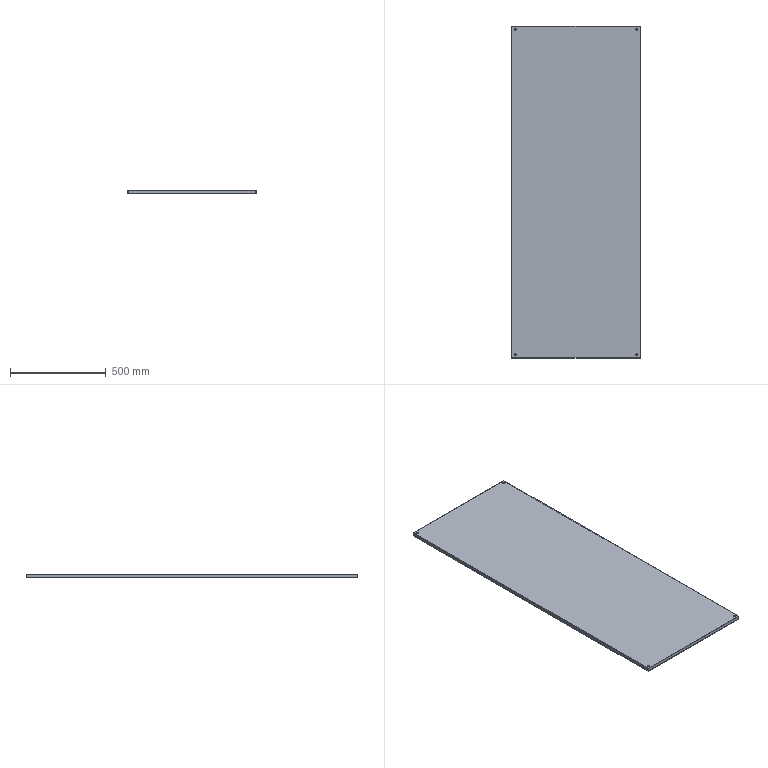Part | SolidWorks | features Extrusion 1, HoleWzd 1, ICE 1, Shell 1 | 1 solid | 32 faces | box 669 x 1734 x 20 mm | volume 2661634 mm3 | cylinder 16 | plane 16 | commonest cylinder face diameters 6.6 x8 11 x8
STEP:
#1=CARTESIAN_POINT('',(-312.,850.,18.));
#2=VERTEX_POINT('',#1);
#3=CARTESIAN_POINT('',(-323.,850.,18.));
#4=VERTEX_POINT('',#3);
#5=CARTESIAN_POINT('',(-317.5,850.,18.));
#6=DIRECTION('',(0.,0.,-1.));
#7=DIRECTION('',(-1.,0.,0.));
#8=AXIS2_PLACEMENT_3D('',#5,#6,#7);
#9=CIRCLE('',#8,5.5);
#10=EDGE_CURVE('',#2,#4,#9,.T.);
#11=ORIENTED_EDGE('',*,*,#10,.T.);
#12=CARTESIAN_POINT('',(-323.,850.,20.));
#13=VERTEX_POINT('',#12);
#14=CARTESIAN_POINT('',(-323.,850.,20.));
#15=DIRECTION('',(0.,0.,1.));
#16=VECTOR('',#15,1000.);
#17=LINE('',#14,#16);
#18=EDGE_CURVE('',#4,#13,#17,.T.);
#19=ORIENTED_EDGE('',*,*,#18,.T.);
#20=CARTESIAN_POINT('',(-312.,850.,20.));
#21=VERTEX_POINT('',#20);
#22=CARTESIAN_POINT('',(-317.5,850.,20.));
#23=DIRECTION('',(0.,0.,1.));
#24=DIRECTION('',(1.,0.,0.));
#25=AXIS2_PLACEMENT_3D('',#22,#23,#24);
#26=CIRCLE('',#25,5.5);
#27=EDGE_CURVE('',#13,#21,#26,.T.);
#28=ORIENTED_EDGE('',*,*,#27,.T.);
#29=CARTESIAN_POINT('',(-312.,850.,20.));
#30=DIRECTION('',(0.,0.,1.));
#31=VECTOR('',#30,1000.);
#32=LINE('',#29,#31);
#33=EDGE_CURVE('',#2,#21,#32,.T.);
#34=ORIENTED_EDGE('',*,*,#33,.F.);
#35=EDGE_LOOP('',(#11,#19,#28,#34));
#36=FACE_OUTER_BOUND('',#35,.T.);
#37=CARTESIAN_POINT('',(-317.5,850.,20.));
#38=DIRECTION('',(0.,0.,1.));
#39=DIRECTION('',(1.,0.,0.));
#40=AXIS2_PLACEMENT_3D('',#37,#38,#39);
#41=CYLINDRICAL_SURFACE('',#40,5.5);
#42=ADVANCED_FACE('',(#36),#41,.F.);
#43=CARTESIAN_POINT('',(-320.8,850.,0.));
#44=VERTEX_POINT('',#43);
#45=CARTESIAN_POINT('',(-314.2,850.,0.));
#46=VERTEX_POINT('',#45);
#47=CARTESIAN_POINT('',(-317.5,850.,0.));
#48=DIRECTION('',(0.,0.,1.));
#49=DIRECTION('',(1.,0.,0.));
#50=AXIS2_PLACEMENT_3D('',#47,#48,#49);
#51=CIRCLE('',#50,3.3);
#52=EDGE_CURVE('',#44,#46,#51,.T.);
#53=ORIENTED_EDGE('',*,*,#52,.F.);
#54=CARTESIAN_POINT('',(-320.8,850.,2.));
#55=VERTEX_POINT('',#54);
#56=CARTESIAN_POINT('',(-320.8,850.,20.));
#57=DIRECTION('',(0.,0.,1.));
#58=VECTOR('',#57,1000.);
#59=LINE('',#56,#58);
#60=EDGE_CURVE('',#44,#55,#59,.T.);
#61=ORIENTED_EDGE('',*,*,#60,.T.);
#62=CARTESIAN_POINT('',(-314.2,850.,2.));
#63=VERTEX_POINT('',#62);
#64=CARTESIAN_POINT('',(-317.5,850.,2.));
#65=DIRECTION('',(0.,0.,-1.));
#66=DIRECTION('',(-1.,0.,0.));
#67=AXIS2_PLACEMENT_3D('',#64,#65,#66);
#68=CIRCLE('',#67,3.3);
#69=EDGE_CURVE('',#63,#55,#68,.T.);
#70=ORIENTED_EDGE('',*,*,#69,.F.);
#71=CARTESIAN_POINT('',(-314.2,850.,20.));
#72=DIRECTION('',(0.,0.,1.));
#73=VECTOR('',#72,1000.);
#74=LINE('',#71,#73);
#75=EDGE_CURVE('',#46,#63,#74,.T.);
#76=ORIENTED_EDGE('',*,*,#75,.F.);
#77=EDGE_LOOP('',(#53,#61,#70,#76));
#78=FACE_OUTER_BOUND('',#77,.T.);
#79=CARTESIAN_POINT('',(-317.5,850.,20.));
#80=DIRECTION('',(0.,0.,1.));
#81=DIRECTION('',(1.,0.,0.));
#82=AXIS2_PLACEMENT_3D('',#79,#80,#81);
#83=CYLINDRICAL_SURFACE('',#82,3.3);
#84=ADVANCED_FACE('',(#78),#83,.F.);
#85=CARTESIAN_POINT('',(-312.,-850.,18.));
#86=VERTEX_POINT('',#85);
#87=CARTESIAN_POINT('',(-323.,-850.,18.));
#88=VERTEX_POINT('',#87);
#89=CARTESIAN_POINT('',(-317.5,-850.,18.));
#90=DIRECTION('',(0.,0.,-1.));
#91=DIRECTION('',(-1.,0.,0.));
#92=AXIS2_PLACEMENT_3D('',#89,#90,#91);
#93=CIRCLE('',#92,5.5);
#94=EDGE_CURVE('',#86,#88,#93,.T.);
#95=ORIENTED_EDGE('',*,*,#94,.T.);
#96=CARTESIAN_POINT('',(-323.,-850.,20.));
#97=VERTEX_POINT('',#96);
#98=CARTESIAN_POINT('',(-323.,-850.,20.));
#99=DIRECTION('',(0.,0.,1.));
#100=VECTOR('',#99,1000.);
#101=LINE('',#98,#100);
#102=EDGE_CURVE('',#88,#97,#101,.T.);
#103=ORIENTED_EDGE('',*,*,#102,.T.);
#104=CARTESIAN_POINT('',(-312.,-850.,20.));
#105=VERTEX_POINT('',#104);
#106=CARTESIAN_POINT('',(-317.5,-850.,20.));
#107=DIRECTION('',(0.,0.,1.));
#108=DIRECTION('',(1.,0.,0.));
#109=AXIS2_PLACEMENT_3D('',#106,#107,#108);
#110=CIRCLE('',#109,5.5);
#111=EDGE_CURVE('',#97,#105,#110,.T.);
#112=ORIENTED_EDGE('',*,*,#111,.T.);
#113=CARTESIAN_POINT('',(-312.,-850.,20.));
#114=DIRECTION('',(0.,0.,1.));
#115=VECTOR('',#114,1000.);
#116=LINE('',#113,#115);
#117=EDGE_CURVE('',#86,#105,#116,.T.);
#118=ORIENTED_EDGE('',*,*,#117,.F.);
#119=EDGE_LOOP('',(#95,#103,#112,#118));
#120=FACE_OUTER_BOUND('',#119,.T.);
#121=CARTESIAN_POINT('',(-317.5,-850.,20.));
#122=DIRECTION('',(0.,0.,1.));
#123=DIRECTION('',(1.,0.,0.));
#124=AXIS2_PLACEMENT_3D('',#121,#122,#123);
#125=CYLINDRICAL_SURFACE('',#124,5.5);
#126=ADVANCED_FACE('',(#120),#125,.F.);
#127=CARTESIAN_POINT('',(-320.8,-850.,0.));
#128=VERTEX_POINT('',#127);
#129=CARTESIAN_POINT('',(-314.2,-850.,0.));
#130=VERTEX_POINT('',#129);
#131=CARTESIAN_POINT('',(-317.5,-850.,0.));
#132=DIRECTION('',(0.,0.,1.));
#133=DIRECTION('',(1.,0.,0.));
#134=AXIS2_PLACEMENT_3D('',#131,#132,#133);
#135=CIRCLE('',#134,3.3);
#136=EDGE_CURVE('',#128,#130,#135,.T.);
#137=ORIENTED_EDGE('',*,*,#136,.F.);
#138=CARTESIAN_POINT('',(-320.8,-850.,2.));
#139=VERTEX_POINT('',#138);
#140=CARTESIAN_POINT('',(-320.8,-850.,20.));
#141=DIRECTION('',(0.,0.,1.));
#142=VECTOR('',#141,1000.);
#143=LINE('',#140,#142);
#144=EDGE_CURVE('',#128,#139,#143,.T.);
#145=ORIENTED_EDGE('',*,*,#144,.T.);
#146=CARTESIAN_POINT('',(-314.2,-850.,2.));
#147=VERTEX_POINT('',#146);
#148=CARTESIAN_POINT('',(-317.5,-850.,2.));
#149=DIRECTION('',(0.,0.,-1.));
#150=DIRECTION('',(-1.,0.,0.));
#151=AXIS2_PLACEMENT_3D('',#148,#149,#150);
#152=CIRCLE('',#151,3.3);
#153=EDGE_CURVE('',#147,#139,#152,.T.);
#154=ORIENTED_EDGE('',*,*,#153,.F.);
#155=CARTESIAN_POINT('',(-314.2,-850.,20.));
#156=DIRECTION('',(0.,0.,1.));
#157=VECTOR('',#156,1000.);
#158=LINE('',#155,#157);
#159=EDGE_CURVE('',#130,#147,#158,.T.);
#160=ORIENTED_EDGE('',*,*,#159,.F.);
#161=EDGE_LOOP('',(#137,#145,#154,#160));
#162=FACE_OUTER_BOUND('',#161,.T.);
#163=CARTESIAN_POINT('',(-317.5,-850.,20.));
#164=DIRECTION('',(0.,0.,1.));
#165=DIRECTION('',(1.,0.,0.));
#166=AXIS2_PLACEMENT_3D('',#163,#164,#165);
#167=CYLINDRICAL_SURFACE('',#166,3.3);
#168=ADVANCED_FACE('',(#162),#167,.F.);
#169=CARTESIAN_POINT('',(314.2,-850.,0.));
#170=VERTEX_POINT('',#169);
#171=CARTESIAN_POINT('',(320.8,-850.,0.));
#172=VERTEX_POINT('',#171);
#173=CARTESIAN_POINT('',(317.5,-850.,0.));
#174=DIRECTION('',(0.,0.,1.));
#175=DIRECTION('',(1.,0.,0.));
#176=AXIS2_PLACEMENT_3D('',#173,#174,#175);
#177=CIRCLE('',#176,3.3);
#178=EDGE_CURVE('',#170,#172,#177,.T.);
#179=ORIENTED_EDGE('',*,*,#178,.F.);
#180=CARTESIAN_POINT('',(314.2,-850.,2.));
#181=VERTEX_POINT('',#180);
#182=CARTESIAN_POINT('',(314.2,-850.,20.));
#183=DIRECTION('',(0.,0.,1.));
#184=VECTOR('',#183,1000.);
#185=LINE('',#182,#184);
#186=EDGE_CURVE('',#170,#181,#185,.T.);
#187=ORIENTED_EDGE('',*,*,#186,.T.);
#188=CARTESIAN_POINT('',(320.8,-850.,2.));
#189=VERTEX_POINT('',#188);
#190=CARTESIAN_POINT('',(317.5,-850.,2.));
#191=DIRECTION('',(0.,0.,-1.));
#192=DIRECTION('',(-1.,0.,0.));
#193=AXIS2_PLACEMENT_3D('',#190,#191,#192);
#194=CIRCLE('',#193,3.3);
#195=EDGE_CURVE('',#189,#181,#194,.T.);
#196=ORIENTED_EDGE('',*,*,#195,.F.);
#197=CARTESIAN_POINT('',(320.8,-850.,20.));
#198=DIRECTION('',(0.,0.,1.));
#199=VECTOR('',#198,1000.);
#200=LINE('',#197,#199);
#201=EDGE_CURVE('',#172,#189,#200,.T.);
#202=ORIENTED_EDGE('',*,*,#201,.F.);
#203=EDGE_LOOP('',(#179,#187,#196,#202));
#204=FACE_OUTER_BOUND('',#203,.T.);
#205=CARTESIAN_POINT('',(317.5,-850.,20.));
#206=DIRECTION('',(0.,0.,1.));
#207=DIRECTION('',(1.,0.,0.));
#208=AXIS2_PLACEMENT_3D('',#205,#206,#207);
#209=CYLINDRICAL_SURFACE('',#208,3.3);
#210=ADVANCED_FACE('',(#204),#209,.F.);
#211=CARTESIAN_POINT('',(323.,-850.,18.));
#212=VERTEX_POINT('',#211);
#213=CARTESIAN_POINT('',(312.,-850.,18.));
#214=VERTEX_POINT('',#213);
#215=CARTESIAN_POINT('',(317.5,-850.,18.));
#216=DIRECTION('',(0.,0.,-1.));
#217=DIRECTION('',(-1.,0.,0.));
#218=AXIS2_PLACEMENT_3D('',#215,#216,#217);
#219=CIRCLE('',#218,5.5);
#220=EDGE_CURVE('',#212,#214,#219,.T.);
#221=ORIENTED_EDGE('',*,*,#220,.T.);
#222=CARTESIAN_POINT('',(312.,-850.,20.));
#223=VERTEX_POINT('',#222);
#224=CARTESIAN_POINT('',(312.,-850.,20.));
#225=DIRECTION('',(0.,0.,1.));
#226=VECTOR('',#225,1000.);
#227=LINE('',#224,#226);
#228=EDGE_CURVE('',#214,#223,#227,.T.);
#229=ORIENTED_EDGE('',*,*,#228,.T.);
#230=CARTESIAN_POINT('',(323.,-850.,20.));
#231=VERTEX_POINT('',#230);
#232=CARTESIAN_POINT('',(317.5,-850.,20.));
#233=DIRECTION('',(0.,0.,1.));
#234=DIRECTION('',(1.,0.,0.));
#235=AXIS2_PLACEMENT_3D('',#232,#233,#234);
#236=CIRCLE('',#235,5.5);
#237=EDGE_CURVE('',#223,#231,#236,.T.);
#238=ORIENTED_EDGE('',*,*,#237,.T.);
#239=CARTESIAN_POINT('',(323.,-850.,20.));
#240=DIRECTION('',(0.,0.,1.));
#241=VECTOR('',#240,1000.);
#242=LINE('',#239,#241);
#243=EDGE_CURVE('',#212,#231,#242,.T.);
#244=ORIENTED_EDGE('',*,*,#243,.F.);
#245=EDGE_LOOP('',(#221,#229,#238,#244));
#246=FACE_OUTER_BOUND('',#245,.T.);
#247=CARTESIAN_POINT('',(317.5,-850.,20.));
#248=DIRECTION('',(0.,0.,1.));
#249=DIRECTION('',(1.,0.,0.));
#250=AXIS2_PLACEMENT_3D('',#247,#248,#249);
#251=CYLINDRICAL_SURFACE('',#250,5.5);
#252=ADVANCED_FACE('',(#246),#251,.F.);
#253=CARTESIAN_POINT('',(314.2,850.,0.));
#254=VERTEX_POINT('',#253);
#255=CARTESIAN_POINT('',(320.8,850.,0.));
#256=VERTEX_POINT('',#255);
#257=CARTESIAN_POINT('',(317.5,850.,0.));
#258=DIRECTION('',(0.,0.,1.));
#259=DIRECTION('',(1.,0.,0.));
#260=AXIS2_PLACEMENT_3D('',#257,#258,#259);
#261=CIRCLE('',#260,3.3);
#262=EDGE_CURVE('',#254,#256,#261,.T.);
#263=ORIENTED_EDGE('',*,*,#262,.F.);
#264=CARTESIAN_POINT('',(314.2,850.,2.));
#265=VERTEX_POINT('',#264);
#266=CARTESIAN_POINT('',(314.2,850.,20.));
#267=DIRECTION('',(0.,0.,1.));
#268=VECTOR('',#267,1000.);
#269=LINE('',#266,#268);
#270=EDGE_CURVE('',#254,#265,#269,.T.);
#271=ORIENTED_EDGE('',*,*,#270,.T.);
#272=CARTESIAN_POINT('',(320.8,850.,2.));
#273=VERTEX_POINT('',#272);
#274=CARTESIAN_POINT('',(317.5,850.,2.));
#275=DIRECTION('',(0.,0.,-1.));
#276=DIRECTION('',(-1.,0.,0.));
#277=AXIS2_PLACEMENT_3D('',#274,#275,#276);
#278=CIRCLE('',#277,3.3);
#279=EDGE_CURVE('',#273,#265,#278,.T.);
#280=ORIENTED_EDGE('',*,*,#279,.F.);
#281=CARTESIAN_POINT('',(320.8,850.,20.));
#282=DIRECTION('',(0.,0.,1.));
#283=VECTOR('',#282,1000.);
#284=LINE('',#281,#283);
#285=EDGE_CURVE('',#256,#273,#284,.T.);
#286=ORIENTED_EDGE('',*,*,#285,.F.);
#287=EDGE_LOOP('',(#263,#271,#280,#286));
#288=FACE_OUTER_BOUND('',#287,.T.);
#289=CARTESIAN_POINT('',(317.5,850.,20.));
#290=DIRECTION('',(0.,0.,1.));
#291=DIRECTION('',(1.,0.,0.));
#292=AXIS2_PLACEMENT_3D('',#289,#290,#291);
#293=CYLINDRICAL_SURFACE('',#292,3.3);
#294=ADVANCED_FACE('',(#288),#293,.F.);
#295=CARTESIAN_POINT('',(323.,850.,18.));
#296=VERTEX_POINT('',#295);
#297=CARTESIAN_POINT('',(312.,850.,18.));
#298=VERTEX_POINT('',#297);
#299=CARTESIAN_POINT('',(317.5,850.,18.));
#300=DIRECTION('',(0.,0.,-1.));
#301=DIRECTION('',(-1.,0.,0.));
#302=AXIS2_PLACEMENT_3D('',#299,#300,#301);
#303=CIRCLE('',#302,5.5);
#304=EDGE_CURVE('',#296,#298,#303,.T.);
#305=ORIENTED_EDGE('',*,*,#304,.T.);
#306=CARTESIAN_POINT('',(312.,850.,20.));
#307=VERTEX_POINT('',#306);
#308=CARTESIAN_POINT('',(312.,850.,20.));
#309=DIRECTION('',(0.,0.,1.));
#310=VECTOR('',#309,1000.);
#311=LINE('',#308,#310);
#312=EDGE_CURVE('',#298,#307,#311,.T.);
#313=ORIENTED_EDGE('',*,*,#312,.T.);
#314=CARTESIAN_POINT('',(323.,850.,20.));
#315=VERTEX_POINT('',#314);
#316=CARTESIAN_POINT('',(317.5,850.,20.));
#317=DIRECTION('',(0.,0.,1.));
#318=DIRECTION('',(1.,0.,0.));
#319=AXIS2_PLACEMENT_3D('',#316,#317,#318);
#320=CIRCLE('',#319,5.5);
#321=EDGE_CURVE('',#307,#315,#320,.T.);
#322=ORIENTED_EDGE('',*,*,#321,.T.);
#323=CARTESIAN_POINT('',(323.,850.,20.));
#324=DIRECTION('',(0.,0.,1.));
#325=VECTOR('',#324,1000.);
#326=LINE('',#323,#325);
#327=EDGE_CURVE('',#296,#315,#326,.T.);
#328=ORIENTED_EDGE('',*,*,#327,.F.);
#329=EDGE_LOOP('',(#305,#313,#322,#328));
#330=FACE_OUTER_BOUND('',#329,.T.);
#331=CARTESIAN_POINT('',(317.5,850.,20.));
#332=DIRECTION('',(0.,0.,1.));
#333=DIRECTION('',(1.,0.,0.));
#334=AXIS2_PLACEMENT_3D('',#331,#332,#333);
#335=CYLINDRICAL_SURFACE('',#334,5.5);
#336=ADVANCED_FACE('',(#330),#335,.F.);
#337=CARTESIAN_POINT('',(-317.5,850.,0.));
#338=DIRECTION('',(0.,0.,1.));
#339=DIRECTION('',(1.,0.,0.));
#340=AXIS2_PLACEMENT_3D('',#337,#338,#339);
#341=CIRCLE('',#340,3.3);
#342=EDGE_CURVE('',#46,#44,#341,.T.);
#343=ORIENTED_EDGE('',*,*,#342,.T.);
#344=ORIENTED_EDGE('',*,*,#52,.T.);
#345=EDGE_LOOP('',(#343,#344));
#346=FACE_BOUND('',#345,.T.);
#347=CARTESIAN_POINT('',(-317.5,-850.,0.));
#348=DIRECTION('',(0.,0.,1.));
#349=DIRECTION('',(1.,0.,0.));
#350=AXIS2_PLACEMENT_3D('',#347,#348,#349);
#351=CIRCLE('',#350,3.3);
#352=EDGE_CURVE('',#130,#128,#351,.T.);
#353=ORIENTED_EDGE('',*,*,#352,.T.);
#354=ORIENTED_EDGE('',*,*,#136,.T.);
#355=EDGE_LOOP('',(#353,#354));
#356=FACE_BOUND('',#355,.T.);
#357=CARTESIAN_POINT('',(317.5,-850.,0.));
#358=DIRECTION('',(0.,0.,1.));
#359=DIRECTION('',(1.,0.,0.));
#360=AXIS2_PLACEMENT_3D('',#357,#358,#359);
#361=CIRCLE('',#360,3.3);
#362=EDGE_CURVE('',#172,#170,#361,.T.);
#363=ORIENTED_EDGE('',*,*,#362,.T.);
#364=ORIENTED_EDGE('',*,*,#178,.T.);
#365=EDGE_LOOP('',(#363,#364));
#366=FACE_BOUND('',#365,.T.);
#367=CARTESIAN_POINT('',(317.5,850.,0.));
#368=DIRECTION('',(0.,0.,1.));
#369=DIRECTION('',(1.,0.,0.));
#370=AXIS2_PLACEMENT_3D('',#367,#368,#369);
#371=CIRCLE('',#370,3.3);
#372=EDGE_CURVE('',#256,#254,#371,.T.);
#373=ORIENTED_EDGE('',*,*,#372,.T.);
#374=ORIENTED_EDGE('',*,*,#262,.T.);
#375=EDGE_LOOP('',(#373,#374));
#376=FACE_BOUND('',#375,.T.);
#377=CARTESIAN_POINT('',(334.5,-867.,0.));
#378=VERTEX_POINT('',#377);
#379=CARTESIAN_POINT('',(334.5,867.,0.));
#380=VERTEX_POINT('',#379);
#381=CARTESIAN_POINT('',(334.5,-867.,0.));
#382=DIRECTION('',(0.,1.,0.));
#383=VECTOR('',#382,1000.);
#384=LINE('',#381,#383);
#385=EDGE_CURVE('',#378,#380,#384,.T.);
#386=ORIENTED_EDGE('',*,*,#385,.F.);
#387=CARTESIAN_POINT('',(-334.5,-867.,0.));
#388=VERTEX_POINT('',#387);
#389=CARTESIAN_POINT('',(-334.5,-867.,0.));
#390=DIRECTION('',(1.,0.,0.));
#391=VECTOR('',#390,1000.);
#392=LINE('',#389,#391);
#393=EDGE_CURVE('',#388,#378,#392,.T.);
#394=ORIENTED_EDGE('',*,*,#393,.F.);
#395=CARTESIAN_POINT('',(-334.5,867.,0.));
#396=VERTEX_POINT('',#395);
#397=CARTESIAN_POINT('',(-334.5,-867.,0.));
#398=DIRECTION('',(0.,-1.,0.));
#399=VECTOR('',#398,1000.);
#400=LINE('',#397,#399);
#401=EDGE_CURVE('',#396,#388,#400,.T.);
#402=ORIENTED_EDGE('',*,*,#401,.F.);
#403=CARTESIAN_POINT('',(-334.5,867.,0.));
#404=DIRECTION('',(-1.,0.,0.));
#405=VECTOR('',#404,1000.);
#406=LINE('',#403,#405);
#407=EDGE_CURVE('',#380,#396,#406,.T.);
#408=ORIENTED_EDGE('',*,*,#407,.F.);
#409=EDGE_LOOP('',(#386,#394,#402,#408));
#410=FACE_OUTER_BOUND('',#409,.T.);
#411=CARTESIAN_POINT('',(314.5,-847.,0.));
#412=VERTEX_POINT('',#411);
#413=CARTESIAN_POINT('',(-314.5,-847.,0.));
#414=VERTEX_POINT('',#413);
#415=CARTESIAN_POINT('',(314.5,-847.,0.));
#416=DIRECTION('',(-1.,0.,0.));
#417=VECTOR('',#416,1000.);
#418=LINE('',#415,#417);
#419=EDGE_CURVE('',#412,#414,#418,.T.);
#420=ORIENTED_EDGE('',*,*,#419,.F.);
#421=CARTESIAN_POINT('',(314.5,847.,0.));
#422=VERTEX_POINT('',#421);
#423=CARTESIAN_POINT('',(314.5,-847.,0.));
#424=DIRECTION('',(0.,1.,0.));
#425=VECTOR('',#424,1000.);
#426=LINE('',#423,#425);
#427=EDGE_CURVE('',#412,#422,#426,.T.);
#428=ORIENTED_EDGE('',*,*,#427,.T.);
#429=CARTESIAN_POINT('',(-314.5,847.,0.));
#430=VERTEX_POINT('',#429);
#431=CARTESIAN_POINT('',(314.5,847.,0.));
#432=DIRECTION('',(-1.,0.,0.));
#433=VECTOR('',#432,1000.);
#434=LINE('',#431,#433);
#435=EDGE_CURVE('',#422,#430,#434,.T.);
#436=ORIENTED_EDGE('',*,*,#435,.T.);
#437=CARTESIAN_POINT('',(-314.5,-847.,0.));
#438=DIRECTION('',(0.,1.,0.));
#439=VECTOR('',#438,1000.);
#440=LINE('',#437,#439);
#441=EDGE_CURVE('',#414,#430,#440,.T.);
#442=ORIENTED_EDGE('',*,*,#441,.F.);
#443=EDGE_LOOP('',(#420,#428,#436,#442));
#444=FACE_BOUND('',#443,.T.);
#445=CARTESIAN_POINT('',(0.,0.,0.));
#446=DIRECTION('',(0.,0.,-1.));
#447=DIRECTION('',(-1.,0.,0.));
#448=AXIS2_PLACEMENT_3D('',#445,#446,#447);
#449=PLANE('',#448);
#450=ADVANCED_FACE('',(#346,#356,#366,#376,#410,#444),#449,.T.);
#451=ORIENTED_EDGE('',*,*,#385,.T.);
#452=CARTESIAN_POINT('',(334.5,867.,20.));
#453=VERTEX_POINT('',#452);
#454=CARTESIAN_POINT('',(334.5,867.,20.));
#455=DIRECTION('',(0.,0.,-1.));
#456=VECTOR('',#455,1000.);
#457=LINE('',#454,#456);
#458=EDGE_CURVE('',#453,#380,#457,.T.);
#459=ORIENTED_EDGE('',*,*,#458,.F.);
#460=CARTESIAN_POINT('',(334.5,-867.,20.));
#461=VERTEX_POINT('',#460);
#462=CARTESIAN_POINT('',(334.5,-867.,20.));
#463=DIRECTION('',(0.,1.,0.));
#464=VECTOR('',#463,1000.);
#465=LINE('',#462,#464);
#466=EDGE_CURVE('',#461,#453,#465,.T.);
#467=ORIENTED_EDGE('',*,*,#466,.F.);
#468=CARTESIAN_POINT('',(334.5,-867.,20.));
#469=DIRECTION('',(0.,0.,-1.));
#470=VECTOR('',#469,1000.);
#471=LINE('',#468,#470);
#472=EDGE_CURVE('',#461,#378,#471,.T.);
#473=ORIENTED_EDGE('',*,*,#472,.T.);
#474=EDGE_LOOP('',(#451,#459,#467,#473));
#475=FACE_OUTER_BOUND('',#474,.T.);
#476=CARTESIAN_POINT('',(334.5,-867.,20.));
#477=DIRECTION('',(-1.,0.,0.));
#478=DIRECTION('',(0.,0.,1.));
#479=AXIS2_PLACEMENT_3D('',#476,#477,#478);
#480=PLANE('',#479);
#481=ADVANCED_FACE('',(#475),#480,.F.);
#482=ORIENTED_EDGE('',*,*,#407,.T.);
#483=CARTESIAN_POINT('',(-334.5,867.,20.));
#484=VERTEX_POINT('',#483);
#485=CARTESIAN_POINT('',(-334.5,867.,20.));
#486=DIRECTION('',(0.,0.,-1.));
#487=VECTOR('',#486,1000.);
#488=LINE('',#485,#487);
#489=EDGE_CURVE('',#484,#396,#488,.T.);
#490=ORIENTED_EDGE('',*,*,#489,.F.);
#491=CARTESIAN_POINT('',(-334.5,867.,20.));
#492=DIRECTION('',(-1.,0.,0.));
#493=VECTOR('',#492,1000.);
#494=LINE('',#491,#493);
#495=EDGE_CURVE('',#453,#484,#494,.T.);
#496=ORIENTED_EDGE('',*,*,#495,.F.);
#497=ORIENTED_EDGE('',*,*,#458,.T.);
#498=EDGE_LOOP('',(#482,#490,#496,#497));
#499=FACE_OUTER_BOUND('',#498,.T.);
#500=CARTESIAN_POINT('',(-334.5,867.,20.));
#501=DIRECTION('',(0.,-1.,0.));
#502=DIRECTION('',(0.,0.,-1.));
#503=AXIS2_PLACEMENT_3D('',#500,#501,#502);
#504=PLANE('',#503);
#505=ADVANCED_FACE('',(#499),#504,.F.);
#506=ORIENTED_EDGE('',*,*,#401,.T.);
#507=CARTESIAN_POINT('',(-334.5,-867.,20.));
#508=VERTEX_POINT('',#507);
#509=CARTESIAN_POINT('',(-334.5,-867.,20.));
#510=DIRECTION('',(0.,0.,-1.));
#511=VECTOR('',#510,1000.);
#512=LINE('',#509,#511);
#513=EDGE_CURVE('',#508,#388,#512,.T.);
#514=ORIENTED_EDGE('',*,*,#513,.F.);
#515=CARTESIAN_POINT('',(-334.5,-867.,20.));
#516=DIRECTION('',(0.,-1.,0.));
#517=VECTOR('',#516,1000.);
#518=LINE('',#515,#517);
#519=EDGE_CURVE('',#484,#508,#518,.T.);
#520=ORIENTED_EDGE('',*,*,#519,.F.);
#521=ORIENTED_EDGE('',*,*,#489,.T.);
#522=EDGE_LOOP('',(#506,#514,#520,#521));
#523=FACE_OUTER_BOUND('',#522,.T.);
#524=CARTESIAN_POINT('',(-334.5,-867.,20.));
#525=DIRECTION('',(1.,0.,0.));
#526=DIRECTION('',(0.,0.,-1.));
#527=AXIS2_PLACEMENT_3D('',#524,#525,#526);
#528=PLANE('',#527);
#529=ADVANCED_FACE('',(#523),#528,.F.);
#530=ORIENTED_EDGE('',*,*,#393,.T.);
#531=ORIENTED_EDGE('',*,*,#472,.F.);
#532=CARTESIAN_POINT('',(-334.5,-867.,20.));
#533=DIRECTION('',(1.,0.,0.));
#534=VECTOR('',#533,1000.);
#535=LINE('',#532,#534);
#536=EDGE_CURVE('',#508,#461,#535,.T.);
#537=ORIENTED_EDGE('',*,*,#536,.F.);
#538=ORIENTED_EDGE('',*,*,#513,.T.);
#539=EDGE_LOOP('',(#530,#531,#537,#538));
#540=FACE_OUTER_BOUND('',#539,.T.);
#541=CARTESIAN_POINT('',(-334.5,-867.,20.));
#542=DIRECTION('',(0.,1.,0.));
#543=DIRECTION('',(0.,0.,1.));
#544=AXIS2_PLACEMENT_3D('',#541,#542,#543);
#545=PLANE('',#544);
#546=ADVANCED_FACE('',(#540),#545,.F.);
#547=CARTESIAN_POINT('',(-317.5,850.,20.));
#548=DIRECTION('',(0.,0.,1.));
#549=DIRECTION('',(1.,0.,0.));
#550=AXIS2_PLACEMENT_3D('',#547,#548,#549);
#551=CIRCLE('',#550,5.5);
#552=EDGE_CURVE('',#21,#13,#551,.T.);
#553=ORIENTED_EDGE('',*,*,#552,.F.);
#554=ORIENTED_EDGE('',*,*,#27,.F.);
#555=EDGE_LOOP('',(#553,#554));
#556=FACE_BOUND('',#555,.T.);
#557=CARTESIAN_POINT('',(-317.5,-850.,20.));
#558=DIRECTION('',(0.,0.,1.));
#559=DIRECTION('',(1.,0.,0.));
#560=AXIS2_PLACEMENT_3D('',#557,#558,#559);
#561=CIRCLE('',#560,5.5);
#562=EDGE_CURVE('',#105,#97,#561,.T.);
#563=ORIENTED_EDGE('',*,*,#562,.F.);
#564=ORIENTED_EDGE('',*,*,#111,.F.);
#565=EDGE_LOOP('',(#563,#564));
#566=FACE_BOUND('',#565,.T.);
#567=CARTESIAN_POINT('',(317.5,-850.,20.));
#568=DIRECTION('',(0.,0.,1.));
#569=DIRECTION('',(1.,0.,0.));
#570=AXIS2_PLACEMENT_3D('',#567,#568,#569);
#571=CIRCLE('',#570,5.5);
#572=EDGE_CURVE('',#231,#223,#571,.T.);
#573=ORIENTED_EDGE('',*,*,#572,.F.);
#574=ORIENTED_EDGE('',*,*,#237,.F.);
#575=EDGE_LOOP('',(#573,#574));
#576=FACE_BOUND('',#575,.T.);
#577=CARTESIAN_POINT('',(317.5,850.,20.));
#578=DIRECTION('',(0.,0.,1.));
#579=DIRECTION('',(1.,0.,0.));
#580=AXIS2_PLACEMENT_3D('',#577,#578,#579);
#581=CIRCLE('',#580,5.5);
#582=EDGE_CURVE('',#315,#307,#581,.T.);
#583=ORIENTED_EDGE('',*,*,#582,.F.);
#584=ORIENTED_EDGE('',*,*,#321,.F.);
#585=EDGE_LOOP('',(#583,#584));
#586=FACE_BOUND('',#585,.T.);
#587=ORIENTED_EDGE('',*,*,#466,.T.);
#588=ORIENTED_EDGE('',*,*,#495,.T.);
#589=ORIENTED_EDGE('',*,*,#519,.T.);
#590=ORIENTED_EDGE('',*,*,#536,.T.);
#591=EDGE_LOOP('',(#587,#588,#589,#590));
#592=FACE_OUTER_BOUND('',#591,.T.);
#593=CARTESIAN_POINT('',(0.,0.,20.));
#594=DIRECTION('',(0.,0.,-1.));
#595=DIRECTION('',(-1.,0.,0.));
#596=AXIS2_PLACEMENT_3D('',#593,#594,#595);
#597=PLANE('',#596);
#598=ADVANCED_FACE('',(#556,#566,#576,#586,#592),#597,.F.);
#599=ORIENTED_EDGE('',*,*,#427,.F.);
#600=CARTESIAN_POINT('',(314.5,-847.,2.));
#601=VERTEX_POINT('',#600);
#602=CARTESIAN_POINT('',(314.5,-847.,2.));
#603=DIRECTION('',(0.,0.,-1.));
#604=VECTOR('',#603,1000.);
#605=LINE('',#602,#604);
#606=EDGE_CURVE('',#601,#412,#605,.T.);
#607=ORIENTED_EDGE('',*,*,#606,.F.);
#608=CARTESIAN_POINT('',(314.5,847.,2.));
#609=VERTEX_POINT('',#608);
#610=CARTESIAN_POINT('',(314.5,-847.,2.));
#611=DIRECTION('',(0.,1.,0.));
#612=VECTOR('',#611,1000.);
#613=LINE('',#610,#612);
#614=EDGE_CURVE('',#601,#609,#613,.T.);
#615=ORIENTED_EDGE('',*,*,#614,.T.);
#616=CARTESIAN_POINT('',(314.5,847.,2.));
#617=DIRECTION('',(0.,0.,-1.));
#618=VECTOR('',#617,1000.);
#619=LINE('',#616,#618);
#620=EDGE_CURVE('',#609,#422,#619,.T.);
#621=ORIENTED_EDGE('',*,*,#620,.T.);
#622=EDGE_LOOP('',(#599,#607,#615,#621));
#623=FACE_OUTER_BOUND('',#622,.T.);
#624=CARTESIAN_POINT('',(314.5,-847.,2.));
#625=DIRECTION('',(-1.,0.,0.));
#626=DIRECTION('',(0.,0.,1.));
#627=AXIS2_PLACEMENT_3D('',#624,#625,#626);
#628=PLANE('',#627);
#629=ADVANCED_FACE('',(#623),#628,.T.);
#630=ORIENTED_EDGE('',*,*,#435,.F.);
#631=ORIENTED_EDGE('',*,*,#620,.F.);
#632=CARTESIAN_POINT('',(-314.5,847.,2.));
#633=VERTEX_POINT('',#632);
#634=CARTESIAN_POINT('',(314.5,847.,2.));
#635=DIRECTION('',(-1.,0.,0.));
#636=VECTOR('',#635,1000.);
#637=LINE('',#634,#636);
#638=EDGE_CURVE('',#609,#633,#637,.T.);
#639=ORIENTED_EDGE('',*,*,#638,.T.);
#640=CARTESIAN_POINT('',(-314.5,847.,2.));
#641=DIRECTION('',(0.,0.,-1.));
#642=VECTOR('',#641,1000.);
#643=LINE('',#640,#642);
#644=EDGE_CURVE('',#633,#430,#643,.T.);
#645=ORIENTED_EDGE('',*,*,#644,.T.);
#646=EDGE_LOOP('',(#630,#631,#639,#645));
#647=FACE_OUTER_BOUND('',#646,.T.);
#648=CARTESIAN_POINT('',(314.5,847.,2.));
#649=DIRECTION('',(0.,-1.,0.));
#650=DIRECTION('',(0.,0.,-1.));
#651=AXIS2_PLACEMENT_3D('',#648,#649,#650);
#652=PLANE('',#651);
#653=ADVANCED_FACE('',(#647),#652,.T.);
#654=ORIENTED_EDGE('',*,*,#441,.T.);
#655=ORIENTED_EDGE('',*,*,#644,.F.);
#656=CARTESIAN_POINT('',(-314.5,-847.,2.));
#657=VERTEX_POINT('',#656);
#658=CARTESIAN_POINT('',(-314.5,-847.,2.));
#659=DIRECTION('',(0.,1.,0.));
#660=VECTOR('',#659,1000.);
#661=LINE('',#658,#660);
#662=EDGE_CURVE('',#657,#633,#661,.T.);
#663=ORIENTED_EDGE('',*,*,#662,.F.);
#664=CARTESIAN_POINT('',(-314.5,-847.,2.));
#665=DIRECTION('',(0.,0.,-1.));
#666=VECTOR('',#665,1000.);
#667=LINE('',#664,#666);
#668=EDGE_CURVE('',#657,#414,#667,.T.);
#669=ORIENTED_EDGE('',*,*,#668,.T.);
#670=EDGE_LOOP('',(#654,#655,#663,#669));
#671=FACE_OUTER_BOUND('',#670,.T.);
#672=CARTESIAN_POINT('',(-314.5,-847.,2.));
#673=DIRECTION('',(-1.,0.,0.));
#674=DIRECTION('',(0.,0.,1.));
#675=AXIS2_PLACEMENT_3D('',#672,#673,#674);
#676=PLANE('',#675);
#677=ADVANCED_FACE('',(#671),#676,.F.);
#678=ORIENTED_EDGE('',*,*,#419,.T.);
#679=ORIENTED_EDGE('',*,*,#668,.F.);
#680=CARTESIAN_POINT('',(314.5,-847.,2.));
#681=DIRECTION('',(-1.,0.,0.));
#682=VECTOR('',#681,1000.);
#683=LINE('',#680,#682);
#684=EDGE_CURVE('',#601,#657,#683,.T.);
#685=ORIENTED_EDGE('',*,*,#684,.F.);
#686=ORIENTED_EDGE('',*,*,#606,.T.);
#687=EDGE_LOOP('',(#678,#679,#685,#686));
#688=FACE_OUTER_BOUND('',#687,.T.);
#689=CARTESIAN_POINT('',(314.5,-847.,2.));
#690=DIRECTION('',(0.,-1.,0.));
#691=DIRECTION('',(0.,0.,-1.));
#692=AXIS2_PLACEMENT_3D('',#689,#690,#691);
#693=PLANE('',#692);
#694=ADVANCED_FACE('',(#688),#693,.F.);
#695=ORIENTED_EDGE('',*,*,#69,.T.);
#696=CARTESIAN_POINT('',(-317.5,850.,2.));
#697=DIRECTION('',(0.,0.,-1.));
#698=DIRECTION('',(-1.,0.,0.));
#699=AXIS2_PLACEMENT_3D('',#696,#697,#698);
#700=CIRCLE('',#699,3.3);
#701=EDGE_CURVE('',#55,#63,#700,.T.);
#702=ORIENTED_EDGE('',*,*,#701,.T.);
#703=EDGE_LOOP('',(#695,#702));
#704=FACE_BOUND('',#703,.T.);
#705=ORIENTED_EDGE('',*,*,#153,.T.);
#706=CARTESIAN_POINT('',(-317.5,-850.,2.));
#707=DIRECTION('',(0.,0.,-1.));
#708=DIRECTION('',(-1.,0.,0.));
#709=AXIS2_PLACEMENT_3D('',#706,#707,#708);
#710=CIRCLE('',#709,3.3);
#711=EDGE_CURVE('',#139,#147,#710,.T.);
#712=ORIENTED_EDGE('',*,*,#711,.T.);
#713=EDGE_LOOP('',(#705,#712));
#714=FACE_BOUND('',#713,.T.);
#715=ORIENTED_EDGE('',*,*,#195,.T.);
#716=CARTESIAN_POINT('',(317.5,-850.,2.));
#717=DIRECTION('',(0.,0.,-1.));
#718=DIRECTION('',(-1.,0.,0.));
#719=AXIS2_PLACEMENT_3D('',#716,#717,#718);
#720=CIRCLE('',#719,3.3);
#721=EDGE_CURVE('',#181,#189,#720,.T.);
#722=ORIENTED_EDGE('',*,*,#721,.T.);
#723=EDGE_LOOP('',(#715,#722));
#724=FACE_BOUND('',#723,.T.);
#725=ORIENTED_EDGE('',*,*,#279,.T.);
#726=CARTESIAN_POINT('',(317.5,850.,2.));
#727=DIRECTION('',(0.,0.,-1.));
#728=DIRECTION('',(-1.,0.,0.));
#729=AXIS2_PLACEMENT_3D('',#726,#727,#728);
#730=CIRCLE('',#729,3.3);
#731=EDGE_CURVE('',#265,#273,#730,.T.);
#732=ORIENTED_EDGE('',*,*,#731,.T.);
#733=EDGE_LOOP('',(#725,#732));
#734=FACE_BOUND('',#733,.T.);
#735=CARTESIAN_POINT('',(332.5,-865.,2.));
#736=VERTEX_POINT('',#735);
#737=CARTESIAN_POINT('',(332.5,865.,2.));
#738=VERTEX_POINT('',#737);
#739=CARTESIAN_POINT('',(332.5,0.,2.));
#740=DIRECTION('',(0.,1.,0.));
#741=VECTOR('',#740,1000.);
#742=LINE('',#739,#741);
#743=EDGE_CURVE('',#736,#738,#742,.T.);
#744=ORIENTED_EDGE('',*,*,#743,.T.);
#745=CARTESIAN_POINT('',(-332.5,865.,2.));
#746=VERTEX_POINT('',#745);
#747=CARTESIAN_POINT('',(0.,865.,2.));
#748=DIRECTION('',(-1.,0.,0.));
#749=VECTOR('',#748,1000.);
#750=LINE('',#747,#749);
#751=EDGE_CURVE('',#738,#746,#750,.T.);
#752=ORIENTED_EDGE('',*,*,#751,.T.);
#753=CARTESIAN_POINT('',(-332.5,-865.,2.));
#754=VERTEX_POINT('',#753);
#755=CARTESIAN_POINT('',(-332.5,0.,2.));
#756=DIRECTION('',(0.,-1.,0.));
#757=VECTOR('',#756,1000.);
#758=LINE('',#755,#757);
#759=EDGE_CURVE('',#746,#754,#758,.T.);
#760=ORIENTED_EDGE('',*,*,#759,.T.);
#761=CARTESIAN_POINT('',(0.,-865.,2.));
#762=DIRECTION('',(1.,0.,0.));
#763=VECTOR('',#762,1000.);
#764=LINE('',#761,#763);
#765=EDGE_CURVE('',#754,#736,#764,.T.);
#766=ORIENTED_EDGE('',*,*,#765,.T.);
#767=EDGE_LOOP('',(#744,#752,#760,#766));
#768=FACE_OUTER_BOUND('',#767,.T.);
#769=ORIENTED_EDGE('',*,*,#684,.T.);
#770=ORIENTED_EDGE('',*,*,#662,.T.);
#771=ORIENTED_EDGE('',*,*,#638,.F.);
#772=ORIENTED_EDGE('',*,*,#614,.F.);
#773=EDGE_LOOP('',(#769,#770,#771,#772));
#774=FACE_BOUND('',#773,.T.);
#775=CARTESIAN_POINT('',(0.,0.,2.));
#776=DIRECTION('',(0.,0.,-1.));
#777=DIRECTION('',(-1.,0.,0.));
#778=AXIS2_PLACEMENT_3D('',#775,#776,#777);
#779=PLANE('',#778);
#780=ADVANCED_FACE('',(#704,#714,#724,#734,#768,#774),#779,.F.);
#781=ORIENTED_EDGE('',*,*,#743,.F.);
#782=CARTESIAN_POINT('',(332.5,-865.,18.));
#783=VERTEX_POINT('',#782);
#784=CARTESIAN_POINT('',(332.5,-865.,20.));
#785=DIRECTION('',(0.,0.,-1.));
#786=VECTOR('',#785,1000.);
#787=LINE('',#784,#786);
#788=EDGE_CURVE('',#783,#736,#787,.T.);
#789=ORIENTED_EDGE('',*,*,#788,.F.);
#790=CARTESIAN_POINT('',(332.5,865.,18.));
#791=VERTEX_POINT('',#790);
#792=CARTESIAN_POINT('',(332.5,0.,18.));
#793=DIRECTION('',(0.,1.,0.));
#794=VECTOR('',#793,1000.);
#795=LINE('',#792,#794);
#796=EDGE_CURVE('',#783,#791,#795,.T.);
#797=ORIENTED_EDGE('',*,*,#796,.T.);
#798=CARTESIAN_POINT('',(332.5,865.,20.));
#799=DIRECTION('',(0.,0.,-1.));
#800=VECTOR('',#799,1000.);
#801=LINE('',#798,#800);
#802=EDGE_CURVE('',#791,#738,#801,.T.);
#803=ORIENTED_EDGE('',*,*,#802,.T.);
#804=EDGE_LOOP('',(#781,#789,#797,#803));
#805=FACE_OUTER_BOUND('',#804,.T.);
#806=CARTESIAN_POINT('',(332.5,-867.,20.));
#807=DIRECTION('',(-1.,0.,0.));
#808=DIRECTION('',(0.,0.,1.));
#809=AXIS2_PLACEMENT_3D('',#806,#807,#808);
#810=PLANE('',#809);
#811=ADVANCED_FACE('',(#805),#810,.T.);
#812=ORIENTED_EDGE('',*,*,#751,.F.);
#813=ORIENTED_EDGE('',*,*,#802,.F.);
#814=CARTESIAN_POINT('',(-332.5,865.,18.));
#815=VERTEX_POINT('',#814);
#816=CARTESIAN_POINT('',(0.,865.,18.));
#817=DIRECTION('',(-1.,0.,0.));
#818=VECTOR('',#817,1000.);
#819=LINE('',#816,#818);
#820=EDGE_CURVE('',#791,#815,#819,.T.);
#821=ORIENTED_EDGE('',*,*,#820,.T.);
#822=CARTESIAN_POINT('',(-332.5,865.,20.));
#823=DIRECTION('',(0.,0.,-1.));
#824=VECTOR('',#823,1000.);
#825=LINE('',#822,#824);
#826=EDGE_CURVE('',#815,#746,#825,.T.);
#827=ORIENTED_EDGE('',*,*,#826,.T.);
#828=EDGE_LOOP('',(#812,#813,#821,#827));
#829=FACE_OUTER_BOUND('',#828,.T.);
#830=CARTESIAN_POINT('',(-334.5,865.,20.));
#831=DIRECTION('',(0.,-1.,0.));
#832=DIRECTION('',(0.,0.,-1.));
#833=AXIS2_PLACEMENT_3D('',#830,#831,#832);
#834=PLANE('',#833);
#835=ADVANCED_FACE('',(#829),#834,.T.);
#836=ORIENTED_EDGE('',*,*,#759,.F.);
#837=ORIENTED_EDGE('',*,*,#826,.F.);
#838=CARTESIAN_POINT('',(-332.5,-865.,18.));
#839=VERTEX_POINT('',#838);
#840=CARTESIAN_POINT('',(-332.5,0.,18.));
#841=DIRECTION('',(0.,-1.,0.));
#842=VECTOR('',#841,1000.);
#843=LINE('',#840,#842);
#844=EDGE_CURVE('',#815,#839,#843,.T.);
#845=ORIENTED_EDGE('',*,*,#844,.T.);
#846=CARTESIAN_POINT('',(-332.5,-865.,20.));
#847=DIRECTION('',(0.,0.,-1.));
#848=VECTOR('',#847,1000.);
#849=LINE('',#846,#848);
#850=EDGE_CURVE('',#839,#754,#849,.T.);
#851=ORIENTED_EDGE('',*,*,#850,.T.);
#852=EDGE_LOOP('',(#836,#837,#845,#851));
#853=FACE_OUTER_BOUND('',#852,.T.);
#854=CARTESIAN_POINT('',(-332.5,-867.,20.));
#855=DIRECTION('',(1.,0.,0.));
#856=DIRECTION('',(0.,0.,-1.));
#857=AXIS2_PLACEMENT_3D('',#854,#855,#856);
#858=PLANE('',#857);
#859=ADVANCED_FACE('',(#853),#858,.T.);
#860=ORIENTED_EDGE('',*,*,#765,.F.);
#861=ORIENTED_EDGE('',*,*,#850,.F.);
#862=CARTESIAN_POINT('',(0.,-865.,18.));
#863=DIRECTION('',(1.,0.,0.));
#864=VECTOR('',#863,1000.);
#865=LINE('',#862,#864);
#866=EDGE_CURVE('',#839,#783,#865,.T.);
#867=ORIENTED_EDGE('',*,*,#866,.T.);
#868=ORIENTED_EDGE('',*,*,#788,.T.);
#869=EDGE_LOOP('',(#860,#861,#867,#868));
#870=FACE_OUTER_BOUND('',#869,.T.);
#871=CARTESIAN_POINT('',(-334.5,-865.,20.));
#872=DIRECTION('',(0.,1.,0.));
#873=DIRECTION('',(0.,0.,1.));
#874=AXIS2_PLACEMENT_3D('',#871,#872,#873);
#875=PLANE('',#874);
#876=ADVANCED_FACE('',(#870),#875,.T.);
#877=ORIENTED_EDGE('',*,*,#10,.F.);
#878=CARTESIAN_POINT('',(-317.5,850.,18.));
#879=DIRECTION('',(0.,0.,-1.));
#880=DIRECTION('',(-1.,0.,0.));
#881=AXIS2_PLACEMENT_3D('',#878,#879,#880);
#882=CIRCLE('',#881,5.5);
#883=EDGE_CURVE('',#4,#2,#882,.T.);
#884=ORIENTED_EDGE('',*,*,#883,.F.);
#885=EDGE_LOOP('',(#877,#884));
#886=FACE_BOUND('',#885,.T.);
#887=ORIENTED_EDGE('',*,*,#94,.F.);
#888=CARTESIAN_POINT('',(-317.5,-850.,18.));
#889=DIRECTION('',(0.,0.,-1.));
#890=DIRECTION('',(-1.,0.,0.));
#891=AXIS2_PLACEMENT_3D('',#888,#889,#890);
#892=CIRCLE('',#891,5.5);
#893=EDGE_CURVE('',#88,#86,#892,.T.);
#894=ORIENTED_EDGE('',*,*,#893,.F.);
#895=EDGE_LOOP('',(#887,#894));
#896=FACE_BOUND('',#895,.T.);
#897=ORIENTED_EDGE('',*,*,#220,.F.);
#898=CARTESIAN_POINT('',(317.5,-850.,18.));
#899=DIRECTION('',(0.,0.,-1.));
#900=DIRECTION('',(-1.,0.,0.));
#901=AXIS2_PLACEMENT_3D('',#898,#899,#900);
#902=CIRCLE('',#901,5.5);
#903=EDGE_CURVE('',#214,#212,#902,.T.);
#904=ORIENTED_EDGE('',*,*,#903,.F.);
#905=EDGE_LOOP('',(#897,#904));
#906=FACE_BOUND('',#905,.T.);
#907=ORIENTED_EDGE('',*,*,#304,.F.);
#908=CARTESIAN_POINT('',(317.5,850.,18.));
#909=DIRECTION('',(0.,0.,-1.));
#910=DIRECTION('',(-1.,0.,0.));
#911=AXIS2_PLACEMENT_3D('',#908,#909,#910);
#912=CIRCLE('',#911,5.5);
#913=EDGE_CURVE('',#298,#296,#912,.T.);
#914=ORIENTED_EDGE('',*,*,#913,.F.);
#915=EDGE_LOOP('',(#907,#914));
#916=FACE_BOUND('',#915,.T.);
#917=ORIENTED_EDGE('',*,*,#796,.F.);
#918=ORIENTED_EDGE('',*,*,#866,.F.);
#919=ORIENTED_EDGE('',*,*,#844,.F.);
#920=ORIENTED_EDGE('',*,*,#820,.F.);
#921=EDGE_LOOP('',(#917,#918,#919,#920));
#922=FACE_OUTER_BOUND('',#921,.T.);
#923=CARTESIAN_POINT('',(0.,0.,18.));
#924=DIRECTION('',(0.,0.,-1.));
#925=DIRECTION('',(-1.,0.,0.));
#926=AXIS2_PLACEMENT_3D('',#923,#924,#925);
#927=PLANE('',#926);
#928=ADVANCED_FACE('',(#886,#896,#906,#916,#922),#927,.T.);
#929=ORIENTED_EDGE('',*,*,#312,.F.);
#930=ORIENTED_EDGE('',*,*,#913,.T.);
#931=ORIENTED_EDGE('',*,*,#327,.T.);
#932=ORIENTED_EDGE('',*,*,#582,.T.);
#933=EDGE_LOOP('',(#929,#930,#931,#932));
#934=FACE_OUTER_BOUND('',#933,.T.);
#935=CARTESIAN_POINT('',(317.5,850.,20.));
#936=DIRECTION('',(0.,0.,1.));
#937=DIRECTION('',(1.,0.,0.));
#938=AXIS2_PLACEMENT_3D('',#935,#936,#937);
#939=CYLINDRICAL_SURFACE('',#938,5.5);
#940=ADVANCED_FACE('',(#934),#939,.F.);
#941=ORIENTED_EDGE('',*,*,#270,.F.);
#942=ORIENTED_EDGE('',*,*,#372,.F.);
#943=ORIENTED_EDGE('',*,*,#285,.T.);
#944=ORIENTED_EDGE('',*,*,#731,.F.);
#945=EDGE_LOOP('',(#941,#942,#943,#944));
#946=FACE_OUTER_BOUND('',#945,.T.);
#947=CARTESIAN_POINT('',(317.5,850.,20.));
#948=DIRECTION('',(0.,0.,1.));
#949=DIRECTION('',(1.,0.,0.));
#950=AXIS2_PLACEMENT_3D('',#947,#948,#949);
#951=CYLINDRICAL_SURFACE('',#950,3.3);
#952=ADVANCED_FACE('',(#946),#951,.F.);
#953=ORIENTED_EDGE('',*,*,#228,.F.);
#954=ORIENTED_EDGE('',*,*,#903,.T.);
#955=ORIENTED_EDGE('',*,*,#243,.T.);
#956=ORIENTED_EDGE('',*,*,#572,.T.);
#957=EDGE_LOOP('',(#953,#954,#955,#956));
#958=FACE_OUTER_BOUND('',#957,.T.);
#959=CARTESIAN_POINT('',(317.5,-850.,20.));
#960=DIRECTION('',(0.,0.,1.));
#961=DIRECTION('',(1.,0.,0.));
#962=AXIS2_PLACEMENT_3D('',#959,#960,#961);
#963=CYLINDRICAL_SURFACE('',#962,5.5);
#964=ADVANCED_FACE('',(#958),#963,.F.);
#965=ORIENTED_EDGE('',*,*,#186,.F.);
#966=ORIENTED_EDGE('',*,*,#362,.F.);
#967=ORIENTED_EDGE('',*,*,#201,.T.);
#968=ORIENTED_EDGE('',*,*,#721,.F.);
#969=EDGE_LOOP('',(#965,#966,#967,#968));
#970=FACE_OUTER_BOUND('',#969,.T.);
#971=CARTESIAN_POINT('',(317.5,-850.,20.));
#972=DIRECTION('',(0.,0.,1.));
#973=DIRECTION('',(1.,0.,0.));
#974=AXIS2_PLACEMENT_3D('',#971,#972,#973);
#975=CYLINDRICAL_SURFACE('',#974,3.3);
#976=ADVANCED_FACE('',(#970),#975,.F.);
#977=ORIENTED_EDGE('',*,*,#144,.F.);
#978=ORIENTED_EDGE('',*,*,#352,.F.);
#979=ORIENTED_EDGE('',*,*,#159,.T.);
#980=ORIENTED_EDGE('',*,*,#711,.F.);
#981=EDGE_LOOP('',(#977,#978,#979,#980));
#982=FACE_OUTER_BOUND('',#981,.T.);
#983=CARTESIAN_POINT('',(-317.5,-850.,20.));
#984=DIRECTION('',(0.,0.,1.));
#985=DIRECTION('',(1.,0.,0.));
#986=AXIS2_PLACEMENT_3D('',#983,#984,#985);
#987=CYLINDRICAL_SURFACE('',#986,3.3);
#988=ADVANCED_FACE('',(#982),#987,.F.);
#989=ORIENTED_EDGE('',*,*,#102,.F.);
#990=ORIENTED_EDGE('',*,*,#893,.T.);
#991=ORIENTED_EDGE('',*,*,#117,.T.);
#992=ORIENTED_EDGE('',*,*,#562,.T.);
#993=EDGE_LOOP('',(#989,#990,#991,#992));
#994=FACE_OUTER_BOUND('',#993,.T.);
#995=CARTESIAN_POINT('',(-317.5,-850.,20.));
#996=DIRECTION('',(0.,0.,1.));
#997=DIRECTION('',(1.,0.,0.));
#998=AXIS2_PLACEMENT_3D('',#995,#996,#997);
#999=CYLINDRICAL_SURFACE('',#998,5.5);
#1000=ADVANCED_FACE('',(#994),#999,.F.);
#1001=ORIENTED_EDGE('',*,*,#60,.F.);
#1002=ORIENTED_EDGE('',*,*,#342,.F.);
#1003=ORIENTED_EDGE('',*,*,#75,.T.);
#1004=ORIENTED_EDGE('',*,*,#701,.F.);
#1005=EDGE_LOOP('',(#1001,#1002,#1003,#1004));
#1006=FACE_OUTER_BOUND('',#1005,.T.);
#1007=CARTESIAN_POINT('',(-317.5,850.,20.));
#1008=DIRECTION('',(0.,0.,1.));
#1009=DIRECTION('',(1.,0.,0.));
#1010=AXIS2_PLACEMENT_3D('',#1007,#1008,#1009);
#1011=CYLINDRICAL_SURFACE('',#1010,3.3);
#1012=ADVANCED_FACE('',(#1006),#1011,.F.);
#1013=ORIENTED_EDGE('',*,*,#18,.F.);
#1014=ORIENTED_EDGE('',*,*,#883,.T.);
#1015=ORIENTED_EDGE('',*,*,#33,.T.);
#1016=ORIENTED_EDGE('',*,*,#552,.T.);
#1017=EDGE_LOOP('',(#1013,#1014,#1015,#1016));
#1018=FACE_OUTER_BOUND('',#1017,.T.);
#1019=CARTESIAN_POINT('',(-317.5,850.,20.));
#1020=DIRECTION('',(0.,0.,1.));
#1021=DIRECTION('',(1.,0.,0.));
#1022=AXIS2_PLACEMENT_3D('',#1019,#1020,#1021);
#1023=CYLINDRICAL_SURFACE('',#1022,5.5);
#1024=ADVANCED_FACE('',(#1018),#1023,.F.);
#1025=CLOSED_SHELL('',(#42,#84,#126,#168,#210,#252,#294,#336,#450,#481,#505,#529,#546,#598,#629,#653,#677,#694,#780,#811,#835,#859,#876,#928,#940,#952,#964,#976,#988,#1000,#1012,#1024));
#1026=MANIFOLD_SOLID_BREP('',#1025);
#1027=CARTESIAN_POINT('',(0.,0.,0.));
#1028=DIRECTION('',(0.,0.,1.));
#1029=DIRECTION('',(1.,0.,0.));
#1030=AXIS2_PLACEMENT_3D('',#1027,#1028,#1029);
#1031=(LENGTH_UNIT()NAMED_UNIT(*)SI_UNIT(.MILLI.,.METRE.));
#1032=UNCERTAINTY_MEASURE_WITH_UNIT(LENGTH_MEASURE(0.00001),#1031,'','');
#1033=(NAMED_UNIT(*)PLANE_ANGLE_UNIT()SI_UNIT($,.RADIAN.));
#1034=(NAMED_UNIT(*)SI_UNIT($,.STERADIAN.)SOLID_ANGLE_UNIT());
#1035=(GEOMETRIC_REPRESENTATION_CONTEXT(3)GLOBAL_UNCERTAINTY_ASSIGNED_CONTEXT((#1032))GLOBAL_UNIT_ASSIGNED_CONTEXT((#1031,#1033,#1034))REPRESENTATION_CONTEXT('',''));
#1036=ADVANCED_BREP_SHAPE_REPRESENTATION('',(#1026,#1030),#1035);